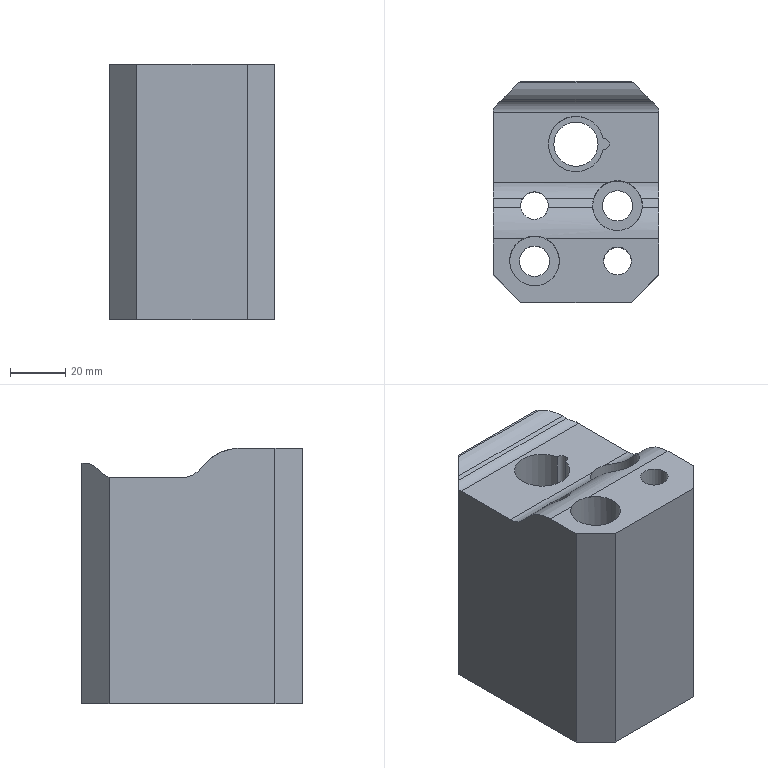Part | NX | features solid 2 | 1 solid | 35 faces | box 60 x 80 x 92.308 mm | volume 320475 mm3 | plane 20 | cylinder 15 | commonest cylinder face diameters 16 x4 10 x3 11 x2 18 x2 4 x1 20 x1
STEP:
#1=CARTESIAN_POINT('',(20.,-440.,5.));
#2=VERTEX_POINT('',#1);
#3=CARTESIAN_POINT('',(20.,-440.,97.308));
#4=VERTEX_POINT('',#3);
#5=CARTESIAN_POINT('',(20.,-440.,10.));
#6=DIRECTION('',(0.,0.,1.));
#7=VECTOR('',#6,1000.);
#8=LINE('',#5,#7);
#9=EDGE_CURVE('',#2,#4,#8,.T.);
#10=ORIENTED_EDGE('',*,*,#9,.T.);
#11=CARTESIAN_POINT('',(-20.,-440.,97.308));
#12=VERTEX_POINT('',#11);
#13=CARTESIAN_POINT('',(0.,-440.,97.308));
#14=DIRECTION('',(-1.,0.,0.));
#15=VECTOR('',#14,1000.);
#16=LINE('',#13,#15);
#17=EDGE_CURVE('',#4,#12,#16,.T.);
#18=ORIENTED_EDGE('',*,*,#17,.T.);
#19=CARTESIAN_POINT('',(-20.,-440.,5.));
#20=VERTEX_POINT('',#19);
#21=CARTESIAN_POINT('',(-20.,-440.,10.));
#22=DIRECTION('',(0.,0.,-1.));
#23=VECTOR('',#22,1000.);
#24=LINE('',#21,#23);
#25=EDGE_CURVE('',#12,#20,#24,.T.);
#26=ORIENTED_EDGE('',*,*,#25,.T.);
#27=CARTESIAN_POINT('',(0.,-440.,5.));
#28=DIRECTION('',(1.,0.,0.));
#29=VECTOR('',#28,1000.);
#30=LINE('',#27,#29);
#31=EDGE_CURVE('',#20,#2,#30,.T.);
#32=ORIENTED_EDGE('',*,*,#31,.T.);
#33=EDGE_LOOP('',(#10,#18,#26,#32));
#34=FACE_BOUND('',#33,.T.);
#35=CARTESIAN_POINT('',(0.,-440.,10.));
#36=DIRECTION('',(0.,-1.,0.));
#37=DIRECTION('',(0.,0.,-1.));
#38=AXIS2_PLACEMENT_3D('',#35,#36,#37);
#39=PLANE('',#38);
#40=ADVANCED_FACE('',(#34),#39,.T.);
#41=CARTESIAN_POINT('',(-20.,-360.,5.));
#42=VERTEX_POINT('',#41);
#43=CARTESIAN_POINT('',(-20.,-360.,92.008));
#44=VERTEX_POINT('',#43);
#45=CARTESIAN_POINT('',(-20.,-360.,10.));
#46=DIRECTION('',(0.,0.,1.));
#47=VECTOR('',#46,1000.);
#48=LINE('',#45,#47);
#49=EDGE_CURVE('',#42,#44,#48,.T.);
#50=ORIENTED_EDGE('',*,*,#49,.T.);
#51=CARTESIAN_POINT('',(20.,-360.,92.008));
#52=VERTEX_POINT('',#51);
#53=CARTESIAN_POINT('',(0.,-360.,92.008));
#54=DIRECTION('',(1.,0.,0.));
#55=VECTOR('',#54,1000.);
#56=LINE('',#53,#55);
#57=EDGE_CURVE('',#44,#52,#56,.T.);
#58=ORIENTED_EDGE('',*,*,#57,.T.);
#59=CARTESIAN_POINT('',(20.,-360.,5.));
#60=VERTEX_POINT('',#59);
#61=CARTESIAN_POINT('',(20.,-360.,10.));
#62=DIRECTION('',(0.,0.,-1.));
#63=VECTOR('',#62,1000.);
#64=LINE('',#61,#63);
#65=EDGE_CURVE('',#52,#60,#64,.T.);
#66=ORIENTED_EDGE('',*,*,#65,.T.);
#67=CARTESIAN_POINT('',(0.,-360.,5.));
#68=DIRECTION('',(-1.,0.,0.));
#69=VECTOR('',#68,1000.);
#70=LINE('',#67,#69);
#71=EDGE_CURVE('',#60,#42,#70,.T.);
#72=ORIENTED_EDGE('',*,*,#71,.T.);
#73=EDGE_LOOP('',(#50,#58,#66,#72));
#74=FACE_BOUND('',#73,.T.);
#75=CARTESIAN_POINT('',(0.,-360.,10.));
#76=DIRECTION('',(0.,1.,0.));
#77=DIRECTION('',(0.,0.,1.));
#78=AXIS2_PLACEMENT_3D('',#75,#76,#77);
#79=PLANE('',#78);
#80=ADVANCED_FACE('',(#74),#79,.T.);
#81=CARTESIAN_POINT('',(30.,-430.,97.308));
#82=VERTEX_POINT('',#81);
#83=CARTESIAN_POINT('',(30.,-430.,5.));
#84=VERTEX_POINT('',#83);
#85=CARTESIAN_POINT('',(30.,-430.,10.));
#86=DIRECTION('',(0.,0.,-1.));
#87=VECTOR('',#86,1000.);
#88=LINE('',#85,#87);
#89=EDGE_CURVE('',#82,#84,#88,.T.);
#90=ORIENTED_EDGE('',*,*,#89,.F.);
#91=CARTESIAN_POINT('',(20.,-440.,97.308));
#92=DIRECTION('',(0.7071,0.7071,0.));
#93=VECTOR('',#92,1000.);
#94=LINE('',#91,#93);
#95=EDGE_CURVE('',#82,#4,#94,.F.);
#96=ORIENTED_EDGE('',*,*,#95,.T.);
#97=ORIENTED_EDGE('',*,*,#9,.F.);
#98=CARTESIAN_POINT('',(50.,-410.,5.));
#99=DIRECTION('',(0.7071,0.7071,0.));
#100=VECTOR('',#99,1000.);
#101=LINE('',#98,#100);
#102=EDGE_CURVE('',#84,#2,#101,.F.);
#103=ORIENTED_EDGE('',*,*,#102,.F.);
#104=EDGE_LOOP('',(#90,#96,#97,#103));
#105=FACE_BOUND('',#104,.T.);
#106=CARTESIAN_POINT('',(20.,-440.,10.));
#107=DIRECTION('',(-0.7071,0.7071,0.));
#108=DIRECTION('',(-0.7071,-0.7071,0.));
#109=AXIS2_PLACEMENT_3D('',#106,#107,#108);
#110=PLANE('',#109);
#111=ADVANCED_FACE('',(#105),#110,.F.);
#112=ORIENTED_EDGE('',*,*,#25,.F.);
#113=CARTESIAN_POINT('',(-30.,-430.,97.308));
#114=VERTEX_POINT('',#113);
#115=CARTESIAN_POINT('',(-30.,-430.,97.308));
#116=DIRECTION('',(0.7071,-0.7071,0.));
#117=VECTOR('',#116,1000.);
#118=LINE('',#115,#117);
#119=EDGE_CURVE('',#12,#114,#118,.F.);
#120=ORIENTED_EDGE('',*,*,#119,.T.);
#121=CARTESIAN_POINT('',(-30.,-430.,5.));
#122=VERTEX_POINT('',#121);
#123=CARTESIAN_POINT('',(-30.,-430.,10.));
#124=DIRECTION('',(0.,0.,1.));
#125=VECTOR('',#124,1000.);
#126=LINE('',#123,#125);
#127=EDGE_CURVE('',#122,#114,#126,.T.);
#128=ORIENTED_EDGE('',*,*,#127,.F.);
#129=CARTESIAN_POINT('',(-50.,-410.,5.));
#130=DIRECTION('',(0.7071,-0.7071,0.));
#131=VECTOR('',#130,1000.);
#132=LINE('',#129,#131);
#133=EDGE_CURVE('',#20,#122,#132,.F.);
#134=ORIENTED_EDGE('',*,*,#133,.F.);
#135=EDGE_LOOP('',(#112,#120,#128,#134));
#136=FACE_BOUND('',#135,.T.);
#137=CARTESIAN_POINT('',(-30.,-430.,10.));
#138=DIRECTION('',(0.7071,0.7071,0.));
#139=DIRECTION('',(-0.7071,0.7071,0.));
#140=AXIS2_PLACEMENT_3D('',#137,#138,#139);
#141=PLANE('',#140);
#142=ADVANCED_FACE('',(#136),#141,.F.);
#143=CARTESIAN_POINT('',(10.,-425.,5.));
#144=VERTEX_POINT('',#143);
#145=CARTESIAN_POINT('',(15.,-425.,5.));
#146=DIRECTION('',(0.,0.,-1.));
#147=DIRECTION('',(-1.,0.,0.));
#148=AXIS2_PLACEMENT_3D('',#145,#146,#147);
#149=CIRCLE('',#148,5.);
#150=EDGE_CURVE('',#144,#144,#149,.T.);
#151=ORIENTED_EDGE('',*,*,#150,.T.);
#152=EDGE_LOOP('',(#151));
#153=FACE_BOUND('',#152,.T.);
#154=CARTESIAN_POINT('',(20.,-425.,97.308));
#155=VERTEX_POINT('',#154);
#156=CARTESIAN_POINT('',(15.,-425.,97.308));
#157=DIRECTION('',(0.,0.,1.));
#158=DIRECTION('',(1.,0.,0.));
#159=AXIS2_PLACEMENT_3D('',#156,#157,#158);
#160=CIRCLE('',#159,5.);
#161=EDGE_CURVE('',#155,#155,#160,.F.);
#162=ORIENTED_EDGE('',*,*,#161,.F.);
#163=EDGE_LOOP('',(#162));
#164=FACE_BOUND('',#163,.T.);
#165=CARTESIAN_POINT('',(15.,-425.,110.));
#166=DIRECTION('',(0.,0.,-1.));
#167=DIRECTION('',(-1.,0.,0.));
#168=AXIS2_PLACEMENT_3D('',#165,#166,#167);
#169=CYLINDRICAL_SURFACE('',#168,5.);
#170=ADVANCED_FACE('',(#153,#164),#169,.F.);
#171=CARTESIAN_POINT('',(-24.,-425.,35.));
#172=VERTEX_POINT('',#171);
#173=CARTESIAN_POINT('',(-15.,-425.,35.));
#174=DIRECTION('',(0.,0.,-1.));
#175=DIRECTION('',(-1.,0.,0.));
#176=AXIS2_PLACEMENT_3D('',#173,#174,#175);
#177=CIRCLE('',#176,9.);
#178=EDGE_CURVE('',#172,#172,#177,.T.);
#179=ORIENTED_EDGE('',*,*,#178,.T.);
#180=EDGE_LOOP('',(#179));
#181=FACE_BOUND('',#180,.T.);
#182=CARTESIAN_POINT('',(-10.799,-417.041,97.308));
#183=VERTEX_POINT('',#182);
#184=CARTESIAN_POINT('',(-19.201,-417.041,97.308));
#185=VERTEX_POINT('',#184);
#186=CARTESIAN_POINT('',(-15.,-425.,97.308));
#187=DIRECTION('',(0.,0.,1.));
#188=DIRECTION('',(1.,0.,0.));
#189=AXIS2_PLACEMENT_3D('',#186,#187,#188);
#190=CIRCLE('',#189,9.);
#191=EDGE_CURVE('',#183,#185,#190,.F.);
#192=ORIENTED_EDGE('',*,*,#191,.F.);
#193=CARTESIAN_POINT('',(-19.201,-417.041,97.308));
#194=CARTESIAN_POINT('',(-17.901,-416.354,97.308));
#195=CARTESIAN_POINT('',(-15.004,-415.646,97.24));
#196=CARTESIAN_POINT('',(-12.099,-416.354,97.308));
#197=CARTESIAN_POINT('',(-10.799,-417.041,97.308));
#198=B_SPLINE_CURVE_WITH_KNOTS('',3,(#193,#194,#195,#196,#197),.UNSPECIFIED.,.F.,.F.,(4,1,4),(0.,0.004347,0.008695),.UNSPECIFIED.);
#199=EDGE_CURVE('',#185,#183,#198,.T.);
#200=ORIENTED_EDGE('',*,*,#199,.F.);
#201=EDGE_LOOP('',(#192,#200));
#202=FACE_BOUND('',#201,.T.);
#203=CARTESIAN_POINT('',(-15.,-425.,110.));
#204=DIRECTION('',(0.,0.,-1.));
#205=DIRECTION('',(-1.,0.,0.));
#206=AXIS2_PLACEMENT_3D('',#203,#204,#205);
#207=CYLINDRICAL_SURFACE('',#206,9.);
#208=ADVANCED_FACE('',(#181,#202),#207,.F.);
#209=CARTESIAN_POINT('',(-30.,-370.,86.857));
#210=VERTEX_POINT('',#209);
#211=CARTESIAN_POINT('',(-30.,-371.212,86.708));
#212=VERTEX_POINT('',#211);
#213=CARTESIAN_POINT('',(-30.,-371.212,91.708));
#214=DIRECTION('',(-1.,0.,0.));
#215=DIRECTION('',(0.,0.,1.));
#216=AXIS2_PLACEMENT_3D('',#213,#214,#215);
#217=CIRCLE('',#216,5.);
#218=EDGE_CURVE('',#210,#212,#217,.T.);
#219=ORIENTED_EDGE('',*,*,#218,.F.);
#220=CARTESIAN_POINT('',(-30.,-370.,5.));
#221=VERTEX_POINT('',#220);
#222=CARTESIAN_POINT('',(-30.,-370.,10.));
#223=DIRECTION('',(0.,0.,-1.));
#224=VECTOR('',#223,1000.);
#225=LINE('',#222,#224);
#226=EDGE_CURVE('',#210,#221,#225,.T.);
#227=ORIENTED_EDGE('',*,*,#226,.T.);
#228=CARTESIAN_POINT('',(-30.,-360.,5.));
#229=DIRECTION('',(0.,-1.,0.));
#230=VECTOR('',#229,1000.);
#231=LINE('',#228,#230);
#232=EDGE_CURVE('',#221,#122,#231,.T.);
#233=ORIENTED_EDGE('',*,*,#232,.T.);
#234=ORIENTED_EDGE('',*,*,#127,.T.);
#235=CARTESIAN_POINT('',(-30.,-417.041,97.308));
#236=VERTEX_POINT('',#235);
#237=CARTESIAN_POINT('',(-30.,-360.,97.308));
#238=DIRECTION('',(0.,1.,0.));
#239=VECTOR('',#238,1000.);
#240=LINE('',#237,#239);
#241=EDGE_CURVE('',#114,#236,#240,.T.);
#242=ORIENTED_EDGE('',*,*,#241,.T.);
#243=CARTESIAN_POINT('',(-30.,-405.652,92.546));
#244=VERTEX_POINT('',#243);
#245=CARTESIAN_POINT('',(-30.,-417.041,81.308));
#246=DIRECTION('',(-1.,0.,0.));
#247=DIRECTION('',(0.,0.,1.));
#248=AXIS2_PLACEMENT_3D('',#245,#246,#247);
#249=CIRCLE('',#248,16.);
#250=EDGE_CURVE('',#236,#244,#249,.T.);
#251=ORIENTED_EDGE('',*,*,#250,.T.);
#252=CARTESIAN_POINT('',(-30.,-402.24,89.089));
#253=VERTEX_POINT('',#252);
#254=CARTESIAN_POINT('',(-30.,-341.861,27.899));
#255=DIRECTION('',(0.,-0.7024,0.7118));
#256=VECTOR('',#255,1000.);
#257=LINE('',#254,#256);
#258=EDGE_CURVE('',#253,#244,#257,.T.);
#259=ORIENTED_EDGE('',*,*,#258,.F.);
#260=CARTESIAN_POINT('',(-30.,-396.546,86.708));
#261=VERTEX_POINT('',#260);
#262=CARTESIAN_POINT('',(-30.,-396.546,94.708));
#263=DIRECTION('',(-1.,0.,0.));
#264=DIRECTION('',(0.,0.,1.));
#265=AXIS2_PLACEMENT_3D('',#262,#263,#264);
#266=CIRCLE('',#265,8.);
#267=EDGE_CURVE('',#261,#253,#266,.T.);
#268=ORIENTED_EDGE('',*,*,#267,.F.);
#269=CARTESIAN_POINT('',(-30.,-360.,86.708));
#270=DIRECTION('',(0.,1.,0.));
#271=VECTOR('',#270,1000.);
#272=LINE('',#269,#271);
#273=EDGE_CURVE('',#261,#212,#272,.T.);
#274=ORIENTED_EDGE('',*,*,#273,.T.);
#275=EDGE_LOOP('',(#219,#227,#233,#234,#242,#251,#259,#268,#274));
#276=FACE_BOUND('',#275,.T.);
#277=CARTESIAN_POINT('',(-30.,-360.,10.));
#278=DIRECTION('',(-1.,0.,0.));
#279=DIRECTION('',(0.,0.,1.));
#280=AXIS2_PLACEMENT_3D('',#277,#278,#279);
#281=PLANE('',#280);
#282=ADVANCED_FACE('',(#276),#281,.T.);
#283=CARTESIAN_POINT('',(-11.511,-382.714,5.));
#284=VERTEX_POINT('',#283);
#285=CARTESIAN_POINT('',(-0.01051,-382.714,5.));
#286=DIRECTION('',(0.,0.,-1.));
#287=DIRECTION('',(-1.,0.,0.));
#288=AXIS2_PLACEMENT_3D('',#285,#286,#287);
#289=CIRCLE('',#288,11.5);
#290=EDGE_CURVE('',#284,#284,#289,.F.);
#291=ORIENTED_EDGE('',*,*,#290,.T.);
#292=EDGE_LOOP('',(#291));
#293=FACE_BOUND('',#292,.T.);
#294=CARTESIAN_POINT('',(9.5,-405.,5.));
#295=VERTEX_POINT('',#294);
#296=CARTESIAN_POINT('',(15.,-405.,5.));
#297=DIRECTION('',(0.,0.,-1.));
#298=DIRECTION('',(-1.,0.,0.));
#299=AXIS2_PLACEMENT_3D('',#296,#297,#298);
#300=CIRCLE('',#299,5.5);
#301=EDGE_CURVE('',#295,#295,#300,.T.);
#302=ORIENTED_EDGE('',*,*,#301,.F.);
#303=EDGE_LOOP('',(#302));
#304=FACE_BOUND('',#303,.T.);
#305=CARTESIAN_POINT('',(-20.5,-425.,5.));
#306=VERTEX_POINT('',#305);
#307=CARTESIAN_POINT('',(-15.,-425.,5.));
#308=DIRECTION('',(0.,0.,-1.));
#309=DIRECTION('',(-1.,0.,0.));
#310=AXIS2_PLACEMENT_3D('',#307,#308,#309);
#311=CIRCLE('',#310,5.5);
#312=EDGE_CURVE('',#306,#306,#311,.T.);
#313=ORIENTED_EDGE('',*,*,#312,.F.);
#314=EDGE_LOOP('',(#313));
#315=FACE_BOUND('',#314,.T.);
#316=CARTESIAN_POINT('',(-20.,-405.,5.));
#317=VERTEX_POINT('',#316);
#318=CARTESIAN_POINT('',(-15.,-405.,5.));
#319=DIRECTION('',(0.,0.,-1.));
#320=DIRECTION('',(-1.,0.,0.));
#321=AXIS2_PLACEMENT_3D('',#318,#319,#320);
#322=CIRCLE('',#321,5.);
#323=EDGE_CURVE('',#317,#317,#322,.T.);
#324=ORIENTED_EDGE('',*,*,#323,.F.);
#325=EDGE_LOOP('',(#324));
#326=FACE_BOUND('',#325,.T.);
#327=ORIENTED_EDGE('',*,*,#150,.F.);
#328=EDGE_LOOP('',(#327));
#329=FACE_BOUND('',#328,.T.);
#330=CARTESIAN_POINT('',(30.,-370.,5.));
#331=VERTEX_POINT('',#330);
#332=CARTESIAN_POINT('',(30.,-360.,5.));
#333=DIRECTION('',(0.,1.,0.));
#334=VECTOR('',#333,1000.);
#335=LINE('',#332,#334);
#336=EDGE_CURVE('',#84,#331,#335,.T.);
#337=ORIENTED_EDGE('',*,*,#336,.F.);
#338=ORIENTED_EDGE('',*,*,#102,.T.);
#339=ORIENTED_EDGE('',*,*,#31,.F.);
#340=ORIENTED_EDGE('',*,*,#133,.T.);
#341=ORIENTED_EDGE('',*,*,#232,.F.);
#342=CARTESIAN_POINT('',(-10.,-350.,5.));
#343=DIRECTION('',(-0.7071,-0.7071,0.));
#344=VECTOR('',#343,1000.);
#345=LINE('',#342,#344);
#346=EDGE_CURVE('',#221,#42,#345,.F.);
#347=ORIENTED_EDGE('',*,*,#346,.T.);
#348=ORIENTED_EDGE('',*,*,#71,.F.);
#349=CARTESIAN_POINT('',(10.,-350.,5.));
#350=DIRECTION('',(-0.7071,0.7071,0.));
#351=VECTOR('',#350,1000.);
#352=LINE('',#349,#351);
#353=EDGE_CURVE('',#60,#331,#352,.F.);
#354=ORIENTED_EDGE('',*,*,#353,.T.);
#355=EDGE_LOOP('',(#337,#338,#339,#340,#341,#347,#348,#354));
#356=FACE_BOUND('',#355,.T.);
#357=CARTESIAN_POINT('',(0.,-360.,5.));
#358=DIRECTION('',(0.,0.,-1.));
#359=DIRECTION('',(-1.,0.,0.));
#360=AXIS2_PLACEMENT_3D('',#357,#358,#359);
#361=PLANE('',#360);
#362=ADVANCED_FACE('',(#293,#304,#315,#326,#329,#356),#361,.T.);
#363=CARTESIAN_POINT('',(30.,-371.212,86.708));
#364=VERTEX_POINT('',#363);
#365=CARTESIAN_POINT('',(30.,-370.,86.857));
#366=VERTEX_POINT('',#365);
#367=CARTESIAN_POINT('',(30.,-371.212,91.708));
#368=DIRECTION('',(1.,0.,0.));
#369=DIRECTION('',(0.,0.,-1.));
#370=AXIS2_PLACEMENT_3D('',#367,#368,#369);
#371=CIRCLE('',#370,5.);
#372=EDGE_CURVE('',#364,#366,#371,.T.);
#373=ORIENTED_EDGE('',*,*,#372,.F.);
#374=CARTESIAN_POINT('',(30.,-396.546,86.708));
#375=VERTEX_POINT('',#374);
#376=CARTESIAN_POINT('',(30.,-360.,86.708));
#377=DIRECTION('',(0.,-1.,0.));
#378=VECTOR('',#377,1000.);
#379=LINE('',#376,#378);
#380=EDGE_CURVE('',#364,#375,#379,.T.);
#381=ORIENTED_EDGE('',*,*,#380,.T.);
#382=CARTESIAN_POINT('',(30.,-402.24,89.089));
#383=VERTEX_POINT('',#382);
#384=CARTESIAN_POINT('',(30.,-396.546,94.708));
#385=DIRECTION('',(1.,0.,0.));
#386=DIRECTION('',(0.,0.,-1.));
#387=AXIS2_PLACEMENT_3D('',#384,#385,#386);
#388=CIRCLE('',#387,8.);
#389=EDGE_CURVE('',#383,#375,#388,.T.);
#390=ORIENTED_EDGE('',*,*,#389,.F.);
#391=CARTESIAN_POINT('',(30.,-405.652,92.546));
#392=VERTEX_POINT('',#391);
#393=CARTESIAN_POINT('',(30.,-341.861,27.899));
#394=DIRECTION('',(0.,0.7024,-0.7118));
#395=VECTOR('',#394,1000.);
#396=LINE('',#393,#395);
#397=EDGE_CURVE('',#392,#383,#396,.T.);
#398=ORIENTED_EDGE('',*,*,#397,.F.);
#399=CARTESIAN_POINT('',(30.,-417.041,97.308));
#400=VERTEX_POINT('',#399);
#401=CARTESIAN_POINT('',(30.,-417.041,81.308));
#402=DIRECTION('',(1.,0.,0.));
#403=DIRECTION('',(0.,0.,-1.));
#404=AXIS2_PLACEMENT_3D('',#401,#402,#403);
#405=CIRCLE('',#404,16.);
#406=EDGE_CURVE('',#392,#400,#405,.T.);
#407=ORIENTED_EDGE('',*,*,#406,.T.);
#408=CARTESIAN_POINT('',(30.,-360.,97.308));
#409=DIRECTION('',(0.,-1.,0.));
#410=VECTOR('',#409,1000.);
#411=LINE('',#408,#410);
#412=EDGE_CURVE('',#400,#82,#411,.T.);
#413=ORIENTED_EDGE('',*,*,#412,.T.);
#414=ORIENTED_EDGE('',*,*,#89,.T.);
#415=ORIENTED_EDGE('',*,*,#336,.T.);
#416=CARTESIAN_POINT('',(30.,-370.,10.));
#417=DIRECTION('',(0.,0.,1.));
#418=VECTOR('',#417,1000.);
#419=LINE('',#416,#418);
#420=EDGE_CURVE('',#331,#366,#419,.T.);
#421=ORIENTED_EDGE('',*,*,#420,.T.);
#422=EDGE_LOOP('',(#373,#381,#390,#398,#407,#413,#414,#415,#421));
#423=FACE_BOUND('',#422,.T.);
#424=CARTESIAN_POINT('',(30.,-360.,10.));
#425=DIRECTION('',(1.,0.,0.));
#426=DIRECTION('',(0.,0.,-1.));
#427=AXIS2_PLACEMENT_3D('',#424,#425,#426);
#428=PLANE('',#427);
#429=ADVANCED_FACE('',(#423),#428,.T.);
#430=CARTESIAN_POINT('',(27.512,-367.512,88.345));
#431=VERTEX_POINT('',#430);
#432=CARTESIAN_POINT('',(31.212,-371.212,91.708));
#433=DIRECTION('',(-0.7071,-0.7071,0.));
#434=DIRECTION('',(-0.7071,0.7071,0.));
#435=AXIS2_PLACEMENT_3D('',#432,#433,#434);
#436=ELLIPSE('',#435,7.071,5.);
#437=EDGE_CURVE('',#366,#431,#436,.F.);
#438=ORIENTED_EDGE('',*,*,#437,.F.);
#439=ORIENTED_EDGE('',*,*,#420,.F.);
#440=ORIENTED_EDGE('',*,*,#353,.F.);
#441=ORIENTED_EDGE('',*,*,#65,.F.);
#442=CARTESIAN_POINT('',(20.643,-360.643,92.008));
#443=VERTEX_POINT('',#442);
#444=CARTESIAN_POINT('',(30.,-370.,92.008));
#445=DIRECTION('',(-0.7071,0.7071,0.));
#446=VECTOR('',#445,1000.);
#447=LINE('',#444,#446);
#448=EDGE_CURVE('',#52,#443,#447,.F.);
#449=ORIENTED_EDGE('',*,*,#448,.T.);
#450=CARTESIAN_POINT('',(26.564,-366.564,89.388));
#451=VERTEX_POINT('',#450);
#452=CARTESIAN_POINT('',(20.643,-360.643,84.008));
#453=DIRECTION('',(-0.7071,-0.7071,0.));
#454=DIRECTION('',(-0.7071,0.7071,0.));
#455=AXIS2_PLACEMENT_3D('',#452,#453,#454);
#456=ELLIPSE('',#455,11.314,8.);
#457=EDGE_CURVE('',#443,#451,#456,.F.);
#458=ORIENTED_EDGE('',*,*,#457,.T.);
#459=CARTESIAN_POINT('',(55.911,-395.911,57.099));
#460=DIRECTION('',(-0.5581,0.5581,0.614));
#461=VECTOR('',#460,1000.);
#462=LINE('',#459,#461);
#463=EDGE_CURVE('',#451,#431,#462,.F.);
#464=ORIENTED_EDGE('',*,*,#463,.T.);
#465=EDGE_LOOP('',(#438,#439,#440,#441,#449,#458,#464));
#466=FACE_BOUND('',#465,.T.);
#467=CARTESIAN_POINT('',(30.,-370.,10.));
#468=DIRECTION('',(-0.7071,-0.7071,0.));
#469=DIRECTION('',(0.7071,-0.7071,0.));
#470=AXIS2_PLACEMENT_3D('',#467,#468,#469);
#471=PLANE('',#470);
#472=ADVANCED_FACE('',(#466),#471,.F.);
#473=CARTESIAN_POINT('',(-27.512,-367.512,88.345));
#474=VERTEX_POINT('',#473);
#475=CARTESIAN_POINT('',(-31.212,-371.212,91.708));
#476=DIRECTION('',(0.7071,-0.7071,0.));
#477=DIRECTION('',(-0.7071,-0.7071,0.));
#478=AXIS2_PLACEMENT_3D('',#475,#476,#477);
#479=ELLIPSE('',#478,7.071,5.);
#480=EDGE_CURVE('',#474,#210,#479,.F.);
#481=ORIENTED_EDGE('',*,*,#480,.F.);
#482=CARTESIAN_POINT('',(-26.564,-366.564,89.388));
#483=VERTEX_POINT('',#482);
#484=CARTESIAN_POINT('',(-49.681,-389.681,63.953));
#485=DIRECTION('',(-0.5581,-0.5581,-0.614));
#486=VECTOR('',#485,1000.);
#487=LINE('',#484,#486);
#488=EDGE_CURVE('',#474,#483,#487,.F.);
#489=ORIENTED_EDGE('',*,*,#488,.T.);
#490=CARTESIAN_POINT('',(-20.643,-360.643,92.008));
#491=VERTEX_POINT('',#490);
#492=CARTESIAN_POINT('',(-20.643,-360.643,84.008));
#493=DIRECTION('',(0.7071,-0.7071,0.));
#494=DIRECTION('',(-0.7071,-0.7071,0.));
#495=AXIS2_PLACEMENT_3D('',#492,#493,#494);
#496=ELLIPSE('',#495,11.314,8.);
#497=EDGE_CURVE('',#483,#491,#496,.F.);
#498=ORIENTED_EDGE('',*,*,#497,.T.);
#499=CARTESIAN_POINT('',(-20.,-360.,92.008));
#500=DIRECTION('',(-0.7071,-0.7071,0.));
#501=VECTOR('',#500,1000.);
#502=LINE('',#499,#501);
#503=EDGE_CURVE('',#491,#44,#502,.F.);
#504=ORIENTED_EDGE('',*,*,#503,.T.);
#505=ORIENTED_EDGE('',*,*,#49,.F.);
#506=ORIENTED_EDGE('',*,*,#346,.F.);
#507=ORIENTED_EDGE('',*,*,#226,.F.);
#508=EDGE_LOOP('',(#481,#489,#498,#504,#505,#506,#507));
#509=FACE_BOUND('',#508,.T.);
#510=CARTESIAN_POINT('',(-20.,-360.,10.));
#511=DIRECTION('',(0.7071,-0.7071,0.));
#512=DIRECTION('',(0.7071,0.7071,0.));
#513=AXIS2_PLACEMENT_3D('',#510,#511,#512);
#514=PLANE('',#513);
#515=ADVANCED_FACE('',(#509),#514,.F.);
#516=CARTESIAN_POINT('',(-10.831,-402.24,89.089));
#517=VERTEX_POINT('',#516);
#518=CARTESIAN_POINT('',(-19.169,-402.24,89.089));
#519=VERTEX_POINT('',#518);
#520=CARTESIAN_POINT('',(-10.831,-402.24,89.089));
#521=CARTESIAN_POINT('',(-11.206,-401.674,88.514));
#522=CARTESIAN_POINT('',(-12.345,-400.5,87.7));
#523=CARTESIAN_POINT('',(-15.,-399.751,87.388));
#524=CARTESIAN_POINT('',(-17.652,-400.498,87.699));
#525=CARTESIAN_POINT('',(-18.794,-401.674,88.514));
#526=CARTESIAN_POINT('',(-19.169,-402.24,89.089));
#527=B_SPLINE_CURVE_WITH_KNOTS('',3,(#520,#521,#522,#523,#524,#525,#526),.UNSPECIFIED.,.F.,.F.,(4,1,1,1,4),(0.,0.002634,0.005268,0.007902,0.01054),.UNSPECIFIED.);
#528=EDGE_CURVE('',#517,#519,#527,.T.);
#529=ORIENTED_EDGE('',*,*,#528,.T.);
#530=CARTESIAN_POINT('',(-19.957,-405.652,92.546));
#531=VERTEX_POINT('',#530);
#532=CARTESIAN_POINT('',(-15.,-405.,91.885));
#533=DIRECTION('',(0.,-0.7118,-0.7024));
#534=DIRECTION('',(0.,0.7024,-0.7118));
#535=AXIS2_PLACEMENT_3D('',#532,#533,#534);
#536=ELLIPSE('',#535,7.119,5.);
#537=EDGE_CURVE('',#519,#531,#536,.F.);
#538=ORIENTED_EDGE('',*,*,#537,.T.);
#539=CARTESIAN_POINT('',(-10.043,-405.652,92.546));
#540=VERTEX_POINT('',#539);
#541=CARTESIAN_POINT('',(-10.043,-405.652,92.546));
#542=CARTESIAN_POINT('',(-10.167,-406.597,93.504));
#543=CARTESIAN_POINT('',(-11.003,-408.762,95.124));
#544=CARTESIAN_POINT('',(-14.989,-410.615,95.949));
#545=CARTESIAN_POINT('',(-18.985,-408.779,95.134));
#546=CARTESIAN_POINT('',(-19.833,-406.599,93.506));
#547=CARTESIAN_POINT('',(-19.957,-405.652,92.546));
#548=B_SPLINE_CURVE_WITH_KNOTS('',3,(#541,#542,#543,#544,#545,#546,#547),.UNSPECIFIED.,.F.,.F.,(4,1,1,1,4),(0.,0.003993,0.007986,0.01198,0.01597),.UNSPECIFIED.);
#549=EDGE_CURVE('',#540,#531,#548,.T.);
#550=ORIENTED_EDGE('',*,*,#549,.F.);
#551=CARTESIAN_POINT('',(-15.,-405.,91.885));
#552=DIRECTION('',(0.,-0.7118,-0.7024));
#553=DIRECTION('',(0.,0.7024,-0.7118));
#554=AXIS2_PLACEMENT_3D('',#551,#552,#553);
#555=ELLIPSE('',#554,7.119,5.);
#556=EDGE_CURVE('',#540,#517,#555,.F.);
#557=ORIENTED_EDGE('',*,*,#556,.T.);
#558=EDGE_LOOP('',(#529,#538,#550,#557));
#559=FACE_BOUND('',#558,.T.);
#560=ORIENTED_EDGE('',*,*,#323,.T.);
#561=EDGE_LOOP('',(#560));
#562=FACE_BOUND('',#561,.T.);
#563=CARTESIAN_POINT('',(-15.,-405.,110.));
#564=DIRECTION('',(0.,0.,-1.));
#565=DIRECTION('',(-1.,0.,0.));
#566=AXIS2_PLACEMENT_3D('',#563,#564,#565);
#567=CYLINDRICAL_SURFACE('',#566,5.);
#568=ADVANCED_FACE('',(#559,#562),#567,.F.);
#569=ORIENTED_EDGE('',*,*,#312,.T.);
#570=EDGE_LOOP('',(#569));
#571=FACE_BOUND('',#570,.T.);
#572=CARTESIAN_POINT('',(-20.5,-425.,35.));
#573=VERTEX_POINT('',#572);
#574=CARTESIAN_POINT('',(-15.,-425.,35.));
#575=DIRECTION('',(0.,0.,-1.));
#576=DIRECTION('',(-1.,0.,0.));
#577=AXIS2_PLACEMENT_3D('',#574,#575,#576);
#578=CIRCLE('',#577,5.5);
#579=EDGE_CURVE('',#573,#573,#578,.T.);
#580=ORIENTED_EDGE('',*,*,#579,.F.);
#581=EDGE_LOOP('',(#580));
#582=FACE_BOUND('',#581,.T.);
#583=CARTESIAN_POINT('',(-15.,-425.,5.));
#584=DIRECTION('',(0.,0.,-1.));
#585=DIRECTION('',(-1.,0.,0.));
#586=AXIS2_PLACEMENT_3D('',#583,#584,#585);
#587=CYLINDRICAL_SURFACE('',#586,5.5);
#588=ADVANCED_FACE('',(#571,#582),#587,.F.);
#589=ORIENTED_EDGE('',*,*,#579,.T.);
#590=EDGE_LOOP('',(#589));
#591=FACE_BOUND('',#590,.T.);
#592=ORIENTED_EDGE('',*,*,#178,.F.);
#593=EDGE_LOOP('',(#592));
#594=FACE_BOUND('',#593,.T.);
#595=CARTESIAN_POINT('',(-15.,-425.,35.));
#596=DIRECTION('',(0.,0.,-1.));
#597=DIRECTION('',(-1.,0.,0.));
#598=AXIS2_PLACEMENT_3D('',#595,#596,#597);
#599=PLANE('',#598);
#600=ADVANCED_FACE('',(#591,#594),#599,.F.);
#601=ORIENTED_EDGE('',*,*,#301,.T.);
#602=EDGE_LOOP('',(#601));
#603=FACE_BOUND('',#602,.T.);
#604=CARTESIAN_POINT('',(9.5,-405.,35.));
#605=VERTEX_POINT('',#604);
#606=CARTESIAN_POINT('',(15.,-405.,35.));
#607=DIRECTION('',(0.,0.,-1.));
#608=DIRECTION('',(-1.,0.,0.));
#609=AXIS2_PLACEMENT_3D('',#606,#607,#608);
#610=CIRCLE('',#609,5.5);
#611=EDGE_CURVE('',#605,#605,#610,.T.);
#612=ORIENTED_EDGE('',*,*,#611,.F.);
#613=EDGE_LOOP('',(#612));
#614=FACE_BOUND('',#613,.T.);
#615=CARTESIAN_POINT('',(15.,-405.,5.));
#616=DIRECTION('',(0.,0.,-1.));
#617=DIRECTION('',(-1.,0.,0.));
#618=AXIS2_PLACEMENT_3D('',#615,#616,#617);
#619=CYLINDRICAL_SURFACE('',#618,5.5);
#620=ADVANCED_FACE('',(#603,#614),#619,.F.);
#621=ORIENTED_EDGE('',*,*,#611,.T.);
#622=EDGE_LOOP('',(#621));
#623=FACE_BOUND('',#622,.T.);
#624=CARTESIAN_POINT('',(6.,-405.,35.));
#625=VERTEX_POINT('',#624);
#626=CARTESIAN_POINT('',(15.,-405.,35.));
#627=DIRECTION('',(0.,0.,-1.));
#628=DIRECTION('',(-1.,0.,0.));
#629=AXIS2_PLACEMENT_3D('',#626,#627,#628);
#630=CIRCLE('',#629,9.);
#631=EDGE_CURVE('',#625,#625,#630,.T.);
#632=ORIENTED_EDGE('',*,*,#631,.F.);
#633=EDGE_LOOP('',(#632));
#634=FACE_BOUND('',#633,.T.);
#635=CARTESIAN_POINT('',(15.,-405.,35.));
#636=DIRECTION('',(0.,0.,-1.));
#637=DIRECTION('',(-1.,0.,0.));
#638=AXIS2_PLACEMENT_3D('',#635,#636,#637);
#639=PLANE('',#638);
#640=ADVANCED_FACE('',(#623,#634),#639,.F.);
#641=CARTESIAN_POINT('',(11.913,-396.546,86.708));
#642=VERTEX_POINT('',#641);
#643=CARTESIAN_POINT('',(18.087,-396.546,86.708));
#644=VERTEX_POINT('',#643);
#645=CARTESIAN_POINT('',(15.,-405.,86.708));
#646=DIRECTION('',(0.,0.,1.));
#647=DIRECTION('',(1.,0.,0.));
#648=AXIS2_PLACEMENT_3D('',#645,#646,#647);
#649=CIRCLE('',#648,9.);
#650=EDGE_CURVE('',#642,#644,#649,.F.);
#651=ORIENTED_EDGE('',*,*,#650,.F.);
#652=CARTESIAN_POINT('',(6.434,-402.24,89.089));
#653=VERTEX_POINT('',#652);
#654=CARTESIAN_POINT('',(11.913,-396.546,86.708));
#655=CARTESIAN_POINT('',(10.531,-397.051,86.708));
#656=CARTESIAN_POINT('',(8.034,-398.754,86.767));
#657=CARTESIAN_POINT('',(6.759,-401.229,88.064));
#658=CARTESIAN_POINT('',(6.434,-402.24,89.089));
#659=B_SPLINE_CURVE_WITH_KNOTS('',3,(#654,#655,#656,#657,#658),.UNSPECIFIED.,.F.,.F.,(4,1,4),(0.,0.004358,0.008716),.UNSPECIFIED.);
#660=EDGE_CURVE('',#642,#653,#659,.T.);
#661=ORIENTED_EDGE('',*,*,#660,.T.);
#662=CARTESIAN_POINT('',(6.024,-405.652,92.546));
#663=VERTEX_POINT('',#662);
#664=CARTESIAN_POINT('',(15.,-405.,91.885));
#665=DIRECTION('',(0.,-0.7118,-0.7024));
#666=DIRECTION('',(0.,0.7024,-0.7118));
#667=AXIS2_PLACEMENT_3D('',#664,#665,#666);
#668=ELLIPSE('',#667,12.814,9.);
#669=EDGE_CURVE('',#653,#663,#668,.F.);
#670=ORIENTED_EDGE('',*,*,#669,.T.);
#671=CARTESIAN_POINT('',(23.976,-405.652,92.546));
#672=VERTEX_POINT('',#671);
#673=CARTESIAN_POINT('',(23.976,-405.652,92.546));
#674=CARTESIAN_POINT('',(23.914,-406.513,93.419));
#675=CARTESIAN_POINT('',(23.527,-408.421,94.941));
#676=CARTESIAN_POINT('',(21.701,-411.359,96.352));
#677=CARTESIAN_POINT('',(18.672,-413.492,96.93));
#678=CARTESIAN_POINT('',(15.017,-414.251,97.058));
#679=CARTESIAN_POINT('',(11.353,-413.503,96.933));
#680=CARTESIAN_POINT('',(8.315,-411.377,96.358));
#681=CARTESIAN_POINT('',(6.476,-408.434,94.95));
#682=CARTESIAN_POINT('',(6.086,-406.514,93.42));
#683=CARTESIAN_POINT('',(6.024,-405.652,92.546));
#684=B_SPLINE_CURVE_WITH_KNOTS('',3,(#673,#674,#675,#676,#677,#678,#679,#680,#681,#682,#683),.UNSPECIFIED.,.F.,.F.,(4,1,1,1,1,1,1,1,4),(0.,0.003639,0.007278,0.01092,0.01456,0.01819,0.02183,0.02547,0.02911),.UNSPECIFIED.);
#685=EDGE_CURVE('',#672,#663,#684,.T.);
#686=ORIENTED_EDGE('',*,*,#685,.F.);
#687=CARTESIAN_POINT('',(23.566,-402.24,89.089));
#688=VERTEX_POINT('',#687);
#689=CARTESIAN_POINT('',(15.,-405.,91.885));
#690=DIRECTION('',(0.,-0.7118,-0.7024));
#691=DIRECTION('',(0.,0.7024,-0.7118));
#692=AXIS2_PLACEMENT_3D('',#689,#690,#691);
#693=ELLIPSE('',#692,12.814,9.);
#694=EDGE_CURVE('',#672,#688,#693,.F.);
#695=ORIENTED_EDGE('',*,*,#694,.T.);
#696=CARTESIAN_POINT('',(23.566,-402.24,89.089));
#697=CARTESIAN_POINT('',(23.242,-401.232,88.067));
#698=CARTESIAN_POINT('',(21.982,-398.77,86.771));
#699=CARTESIAN_POINT('',(19.467,-397.05,86.708));
#700=CARTESIAN_POINT('',(18.087,-396.546,86.708));
#701=B_SPLINE_CURVE_WITH_KNOTS('',3,(#696,#697,#698,#699,#700),.UNSPECIFIED.,.F.,.F.,(4,1,4),(0.,0.004352,0.008704),.UNSPECIFIED.);
#702=EDGE_CURVE('',#688,#644,#701,.T.);
#703=ORIENTED_EDGE('',*,*,#702,.T.);
#704=EDGE_LOOP('',(#651,#661,#670,#686,#695,#703));
#705=FACE_BOUND('',#704,.T.);
#706=ORIENTED_EDGE('',*,*,#631,.T.);
#707=EDGE_LOOP('',(#706));
#708=FACE_BOUND('',#707,.T.);
#709=CARTESIAN_POINT('',(15.,-405.,110.));
#710=DIRECTION('',(0.,0.,-1.));
#711=DIRECTION('',(-1.,0.,0.));
#712=AXIS2_PLACEMENT_3D('',#709,#710,#711);
#713=CYLINDRICAL_SURFACE('',#712,9.);
#714=ADVANCED_FACE('',(#705,#708),#713,.F.);
#715=ORIENTED_EDGE('',*,*,#412,.F.);
#716=CARTESIAN_POINT('',(30.,-417.041,97.308));
#717=CARTESIAN_POINT('',(16.4,-417.041,97.308));
#718=CARTESIAN_POINT('',(2.801,-417.041,97.308));
#719=CARTESIAN_POINT('',(-10.799,-417.041,97.308));
#720=B_SPLINE_CURVE_WITH_KNOTS('',3,(#716,#717,#718,#719),.UNSPECIFIED.,.F.,.F.,(4,4),(0.4635,0.5128),.UNSPECIFIED.);
#721=EDGE_CURVE('',#400,#183,#720,.T.);
#722=ORIENTED_EDGE('',*,*,#721,.T.);
#723=ORIENTED_EDGE('',*,*,#191,.T.);
#724=CARTESIAN_POINT('',(-19.201,-417.041,97.308));
#725=CARTESIAN_POINT('',(-22.801,-417.041,97.308));
#726=CARTESIAN_POINT('',(-26.4,-417.041,97.308));
#727=CARTESIAN_POINT('',(-30.,-417.041,97.308));
#728=B_SPLINE_CURVE_WITH_KNOTS('',3,(#724,#725,#726,#727),.UNSPECIFIED.,.F.,.F.,(4,4),(0.523,0.536),.UNSPECIFIED.);
#729=EDGE_CURVE('',#185,#236,#728,.T.);
#730=ORIENTED_EDGE('',*,*,#729,.T.);
#731=ORIENTED_EDGE('',*,*,#241,.F.);
#732=ORIENTED_EDGE('',*,*,#119,.F.);
#733=ORIENTED_EDGE('',*,*,#17,.F.);
#734=ORIENTED_EDGE('',*,*,#95,.F.);
#735=EDGE_LOOP('',(#715,#722,#723,#730,#731,#732,#733,#734));
#736=FACE_BOUND('',#735,.T.);
#737=ORIENTED_EDGE('',*,*,#161,.T.);
#738=EDGE_LOOP('',(#737));
#739=FACE_BOUND('',#738,.T.);
#740=CARTESIAN_POINT('',(532.124,-754.014,97.308));
#741=DIRECTION('',(0.,0.,1.));
#742=DIRECTION('',(0.,-1.,0.));
#743=AXIS2_PLACEMENT_3D('',#740,#741,#742);
#744=PLANE('',#743);
#745=ADVANCED_FACE('',(#736,#739),#744,.T.);
#746=CARTESIAN_POINT('',(9.789,-384.704,86.708));
#747=VERTEX_POINT('',#746);
#748=CARTESIAN_POINT('',(9.789,-380.724,86.708));
#749=VERTEX_POINT('',#748);
#750=CARTESIAN_POINT('',(9.989,-382.714,86.708));
#751=DIRECTION('',(0.,0.,1.));
#752=DIRECTION('',(1.,0.,0.));
#753=AXIS2_PLACEMENT_3D('',#750,#751,#752);
#754=CIRCLE('',#753,2.);
#755=EDGE_CURVE('',#747,#749,#754,.T.);
#756=ORIENTED_EDGE('',*,*,#755,.F.);
#757=CARTESIAN_POINT('',(-0.01051,-382.714,86.708));
#758=DIRECTION('',(0.,0.,1.));
#759=DIRECTION('',(1.,0.,0.));
#760=AXIS2_PLACEMENT_3D('',#757,#758,#759);
#761=CIRCLE('',#760,10.);
#762=EDGE_CURVE('',#747,#749,#761,.F.);
#763=ORIENTED_EDGE('',*,*,#762,.T.);
#764=EDGE_LOOP('',(#756,#763));
#765=FACE_BOUND('',#764,.T.);
#766=ORIENTED_EDGE('',*,*,#273,.F.);
#767=CARTESIAN_POINT('',(-30.,-396.546,86.708));
#768=CARTESIAN_POINT('',(-16.029,-396.546,86.708));
#769=CARTESIAN_POINT('',(-2.058,-396.546,86.708));
#770=CARTESIAN_POINT('',(11.913,-396.546,86.708));
#771=B_SPLINE_CURVE_WITH_KNOTS('',3,(#767,#768,#769,#770),.UNSPECIFIED.,.F.,.F.,(4,4),(0.464,0.5146),.UNSPECIFIED.);
#772=EDGE_CURVE('',#261,#642,#771,.T.);
#773=ORIENTED_EDGE('',*,*,#772,.T.);
#774=ORIENTED_EDGE('',*,*,#650,.T.);
#775=CARTESIAN_POINT('',(18.087,-396.546,86.708));
#776=CARTESIAN_POINT('',(22.058,-396.546,86.708));
#777=CARTESIAN_POINT('',(26.029,-396.546,86.708));
#778=CARTESIAN_POINT('',(30.,-396.546,86.708));
#779=B_SPLINE_CURVE_WITH_KNOTS('',3,(#775,#776,#777,#778),.UNSPECIFIED.,.F.,.F.,(4,4),(0.5221,0.5365),.UNSPECIFIED.);
#780=EDGE_CURVE('',#644,#375,#779,.T.);
#781=ORIENTED_EDGE('',*,*,#780,.T.);
#782=ORIENTED_EDGE('',*,*,#380,.F.);
#783=CARTESIAN_POINT('',(30.,-371.212,86.708));
#784=CARTESIAN_POINT('',(10.,-371.212,86.708));
#785=CARTESIAN_POINT('',(-10.,-371.212,86.708));
#786=CARTESIAN_POINT('',(-30.,-371.212,86.708));
#787=B_SPLINE_CURVE_WITH_KNOTS('',3,(#783,#784,#785,#786),.UNSPECIFIED.,.F.,.F.,(4,4),(0.273,0.727),.UNSPECIFIED.);
#788=EDGE_CURVE('',#364,#212,#787,.T.);
#789=ORIENTED_EDGE('',*,*,#788,.T.);
#790=EDGE_LOOP('',(#766,#773,#774,#781,#782,#789));
#791=FACE_BOUND('',#790,.T.);
#792=CARTESIAN_POINT('',(426.488,227.578,86.708));
#793=DIRECTION('',(0.,0.,1.));
#794=DIRECTION('',(0.,-1.,0.));
#795=AXIS2_PLACEMENT_3D('',#792,#793,#794);
#796=PLANE('',#795);
#797=ADVANCED_FACE('',(#765,#791),#796,.T.);
#798=ORIENTED_EDGE('',*,*,#250,.F.);
#799=ORIENTED_EDGE('',*,*,#729,.F.);
#800=ORIENTED_EDGE('',*,*,#199,.T.);
#801=ORIENTED_EDGE('',*,*,#721,.F.);
#802=ORIENTED_EDGE('',*,*,#406,.F.);
#803=CARTESIAN_POINT('',(30.,-405.652,92.546));
#804=CARTESIAN_POINT('',(27.992,-405.652,92.546));
#805=CARTESIAN_POINT('',(25.984,-405.652,92.546));
#806=CARTESIAN_POINT('',(23.976,-405.652,92.546));
#807=B_SPLINE_CURVE_WITH_KNOTS('',3,(#803,#804,#805,#806),.UNSPECIFIED.,.F.,.F.,(4,4),(0.4635,0.4708),.UNSPECIFIED.);
#808=EDGE_CURVE('',#672,#392,#807,.F.);
#809=ORIENTED_EDGE('',*,*,#808,.F.);
#810=ORIENTED_EDGE('',*,*,#685,.T.);
#811=CARTESIAN_POINT('',(6.024,-405.652,92.546));
#812=CARTESIAN_POINT('',(0.6682,-405.652,92.546));
#813=CARTESIAN_POINT('',(-4.687,-405.652,92.546));
#814=CARTESIAN_POINT('',(-10.043,-405.652,92.546));
#815=B_SPLINE_CURVE_WITH_KNOTS('',3,(#811,#812,#813,#814),.UNSPECIFIED.,.F.,.F.,(4,4),(0.4925,0.5119),.UNSPECIFIED.);
#816=EDGE_CURVE('',#540,#663,#815,.F.);
#817=ORIENTED_EDGE('',*,*,#816,.F.);
#818=ORIENTED_EDGE('',*,*,#549,.T.);
#819=CARTESIAN_POINT('',(-19.957,-405.652,92.546));
#820=CARTESIAN_POINT('',(-23.305,-405.652,92.546));
#821=CARTESIAN_POINT('',(-26.652,-405.652,92.546));
#822=CARTESIAN_POINT('',(-30.,-405.652,92.546));
#823=B_SPLINE_CURVE_WITH_KNOTS('',3,(#819,#820,#821,#822),.UNSPECIFIED.,.F.,.F.,(4,4),(0.5239,0.536),.UNSPECIFIED.);
#824=EDGE_CURVE('',#244,#531,#823,.F.);
#825=ORIENTED_EDGE('',*,*,#824,.F.);
#826=EDGE_LOOP('',(#798,#799,#800,#801,#802,#809,#810,#817,#818,#825));
#827=FACE_BOUND('',#826,.T.);
#828=CARTESIAN_POINT('',(-6000414.,-417.041,81.308));
#829=DIRECTION('',(1.,0.,0.));
#830=DIRECTION('',(0.,0.,1.));
#831=AXIS2_PLACEMENT_3D('',#828,#829,#830);
#832=CYLINDRICAL_SURFACE('',#831,16.);
#833=ADVANCED_FACE('',(#827),#832,.T.);
#834=ORIENTED_EDGE('',*,*,#772,.F.);
#835=ORIENTED_EDGE('',*,*,#267,.T.);
#836=CARTESIAN_POINT('',(-30.,-402.24,89.089));
#837=CARTESIAN_POINT('',(-26.39,-402.24,89.089));
#838=CARTESIAN_POINT('',(-22.78,-402.24,89.089));
#839=CARTESIAN_POINT('',(-19.169,-402.24,89.089));
#840=B_SPLINE_CURVE_WITH_KNOTS('',3,(#836,#837,#838,#839),.UNSPECIFIED.,.F.,.F.,(4,4),(0.464,0.4771),.UNSPECIFIED.);
#841=EDGE_CURVE('',#253,#519,#840,.T.);
#842=ORIENTED_EDGE('',*,*,#841,.T.);
#843=ORIENTED_EDGE('',*,*,#528,.F.);
#844=CARTESIAN_POINT('',(-10.831,-402.24,89.089));
#845=CARTESIAN_POINT('',(-5.076,-402.24,89.089));
#846=CARTESIAN_POINT('',(0.6788,-402.24,89.089));
#847=CARTESIAN_POINT('',(6.434,-402.24,89.089));
#848=B_SPLINE_CURVE_WITH_KNOTS('',3,(#844,#845,#846,#847),.UNSPECIFIED.,.F.,.F.,(4,4),(0.4871,0.508),.UNSPECIFIED.);
#849=EDGE_CURVE('',#517,#653,#848,.T.);
#850=ORIENTED_EDGE('',*,*,#849,.T.);
#851=ORIENTED_EDGE('',*,*,#660,.F.);
#852=EDGE_LOOP('',(#834,#835,#842,#843,#850,#851));
#853=FACE_BOUND('',#852,.T.);
#854=CARTESIAN_POINT('',(-6000414.,-396.546,94.708));
#855=DIRECTION('',(1.,0.,0.));
#856=DIRECTION('',(0.,0.,1.));
#857=AXIS2_PLACEMENT_3D('',#854,#855,#856);
#858=CYLINDRICAL_SURFACE('',#857,8.);
#859=ADVANCED_FACE('',(#853),#858,.F.);
#860=CARTESIAN_POINT('',(23.566,-402.24,89.089));
#861=CARTESIAN_POINT('',(25.711,-402.24,89.089));
#862=CARTESIAN_POINT('',(27.855,-402.24,89.089));
#863=CARTESIAN_POINT('',(30.,-402.24,89.089));
#864=B_SPLINE_CURVE_WITH_KNOTS('',3,(#860,#861,#862,#863),.UNSPECIFIED.,.F.,.F.,(4,4),(0.5287,0.5365),.UNSPECIFIED.);
#865=EDGE_CURVE('',#688,#383,#864,.T.);
#866=ORIENTED_EDGE('',*,*,#865,.T.);
#867=ORIENTED_EDGE('',*,*,#389,.T.);
#868=ORIENTED_EDGE('',*,*,#780,.F.);
#869=ORIENTED_EDGE('',*,*,#702,.F.);
#870=EDGE_LOOP('',(#866,#867,#868,#869));
#871=FACE_BOUND('',#870,.T.);
#872=CARTESIAN_POINT('',(-6000414.,-396.546,94.708));
#873=DIRECTION('',(1.,0.,0.));
#874=DIRECTION('',(0.,0.,1.));
#875=AXIS2_PLACEMENT_3D('',#872,#873,#874);
#876=CYLINDRICAL_SURFACE('',#875,8.);
#877=ADVANCED_FACE('',(#871),#876,.F.);
#878=ORIENTED_EDGE('',*,*,#841,.F.);
#879=ORIENTED_EDGE('',*,*,#258,.T.);
#880=ORIENTED_EDGE('',*,*,#824,.T.);
#881=ORIENTED_EDGE('',*,*,#537,.F.);
#882=EDGE_LOOP('',(#878,#879,#880,#881));
#883=FACE_BOUND('',#882,.T.);
#884=CARTESIAN_POINT('',(513.762,-332.088,17.996));
#885=DIRECTION('',(0.,-0.7118,-0.7024));
#886=DIRECTION('',(0.,0.7024,-0.7118));
#887=AXIS2_PLACEMENT_3D('',#884,#885,#886);
#888=PLANE('',#887);
#889=ADVANCED_FACE('',(#883),#888,.F.);
#890=ORIENTED_EDGE('',*,*,#556,.F.);
#891=ORIENTED_EDGE('',*,*,#816,.T.);
#892=ORIENTED_EDGE('',*,*,#669,.F.);
#893=ORIENTED_EDGE('',*,*,#849,.F.);
#894=EDGE_LOOP('',(#890,#891,#892,#893));
#895=FACE_BOUND('',#894,.T.);
#896=CARTESIAN_POINT('',(513.762,-332.088,17.996));
#897=DIRECTION('',(0.,-0.7118,-0.7024));
#898=DIRECTION('',(0.,0.7024,-0.7118));
#899=AXIS2_PLACEMENT_3D('',#896,#897,#898);
#900=PLANE('',#899);
#901=ADVANCED_FACE('',(#895),#900,.F.);
#902=ORIENTED_EDGE('',*,*,#808,.T.);
#903=ORIENTED_EDGE('',*,*,#397,.T.);
#904=ORIENTED_EDGE('',*,*,#865,.F.);
#905=ORIENTED_EDGE('',*,*,#694,.F.);
#906=EDGE_LOOP('',(#902,#903,#904,#905));
#907=FACE_BOUND('',#906,.T.);
#908=CARTESIAN_POINT('',(513.762,-332.088,17.996));
#909=DIRECTION('',(0.,-0.7118,-0.7024));
#910=DIRECTION('',(0.,0.7024,-0.7118));
#911=AXIS2_PLACEMENT_3D('',#908,#909,#910);
#912=PLANE('',#911);
#913=ADVANCED_FACE('',(#907),#912,.F.);
#914=ORIENTED_EDGE('',*,*,#448,.F.);
#915=ORIENTED_EDGE('',*,*,#57,.F.);
#916=ORIENTED_EDGE('',*,*,#503,.F.);
#917=CARTESIAN_POINT('',(-20.643,-360.643,92.008));
#918=CARTESIAN_POINT('',(-6.881,-360.643,92.008));
#919=CARTESIAN_POINT('',(6.881,-360.643,92.008));
#920=CARTESIAN_POINT('',(20.643,-360.643,92.008));
#921=B_SPLINE_CURVE_WITH_KNOTS('',3,(#917,#918,#919,#920),.UNSPECIFIED.,.F.,.F.,(4,4),(0.3413,0.6587),.UNSPECIFIED.);
#922=EDGE_CURVE('',#491,#443,#921,.T.);
#923=ORIENTED_EDGE('',*,*,#922,.T.);
#924=EDGE_LOOP('',(#914,#915,#916,#923));
#925=FACE_BOUND('',#924,.T.);
#926=CARTESIAN_POINT('',(575.068,183.357,92.008));
#927=DIRECTION('',(0.,0.,1.));
#928=DIRECTION('',(0.,-1.,0.));
#929=AXIS2_PLACEMENT_3D('',#926,#927,#928);
#930=PLANE('',#929);
#931=ADVANCED_FACE('',(#925),#930,.T.);
#932=ORIENTED_EDGE('',*,*,#457,.F.);
#933=ORIENTED_EDGE('',*,*,#922,.F.);
#934=ORIENTED_EDGE('',*,*,#497,.F.);
#935=CARTESIAN_POINT('',(26.564,-366.564,89.388));
#936=CARTESIAN_POINT('',(8.855,-366.564,89.388));
#937=CARTESIAN_POINT('',(-8.855,-366.564,89.388));
#938=CARTESIAN_POINT('',(-26.564,-366.564,89.388));
#939=B_SPLINE_CURVE_WITH_KNOTS('',3,(#935,#936,#937,#938),.UNSPECIFIED.,.F.,.F.,(4,4),(0.2958,0.7042),.UNSPECIFIED.);
#940=EDGE_CURVE('',#451,#483,#939,.T.);
#941=ORIENTED_EDGE('',*,*,#940,.F.);
#942=EDGE_LOOP('',(#932,#933,#934,#941));
#943=FACE_BOUND('',#942,.T.);
#944=CARTESIAN_POINT('',(6000065.038,-360.643,84.008));
#945=DIRECTION('',(-1.,0.,0.));
#946=DIRECTION('',(0.,0.,-1.));
#947=AXIS2_PLACEMENT_3D('',#944,#945,#946);
#948=CYLINDRICAL_SURFACE('',#947,8.);
#949=ADVANCED_FACE('',(#943),#948,.T.);
#950=ORIENTED_EDGE('',*,*,#463,.F.);
#951=ORIENTED_EDGE('',*,*,#940,.T.);
#952=ORIENTED_EDGE('',*,*,#488,.F.);
#953=CARTESIAN_POINT('',(-27.512,-367.512,88.345));
#954=CARTESIAN_POINT('',(-9.171,-367.512,88.345));
#955=CARTESIAN_POINT('',(9.171,-367.512,88.345));
#956=CARTESIAN_POINT('',(27.512,-367.512,88.345));
#957=B_SPLINE_CURVE_WITH_KNOTS('',3,(#953,#954,#955,#956),.UNSPECIFIED.,.F.,.F.,(4,4),(0.2918,0.7082),.UNSPECIFIED.);
#958=EDGE_CURVE('',#431,#474,#957,.F.);
#959=ORIENTED_EDGE('',*,*,#958,.F.);
#960=EDGE_LOOP('',(#950,#951,#952,#959));
#961=FACE_BOUND('',#960,.T.);
#962=CARTESIAN_POINT('',(207.327,-359.884,96.738));
#963=DIRECTION('',(0.,-0.74,0.6726));
#964=DIRECTION('',(0.,-0.6726,-0.74));
#965=AXIS2_PLACEMENT_3D('',#962,#963,#964);
#966=PLANE('',#965);
#967=ADVANCED_FACE('',(#961),#966,.T.);
#968=ORIENTED_EDGE('',*,*,#788,.F.);
#969=ORIENTED_EDGE('',*,*,#372,.T.);
#970=ORIENTED_EDGE('',*,*,#437,.T.);
#971=ORIENTED_EDGE('',*,*,#958,.T.);
#972=ORIENTED_EDGE('',*,*,#480,.T.);
#973=ORIENTED_EDGE('',*,*,#218,.T.);
#974=EDGE_LOOP('',(#968,#969,#970,#971,#972,#973));
#975=FACE_BOUND('',#974,.T.);
#976=CARTESIAN_POINT('',(6000066.082,-371.212,91.708));
#977=DIRECTION('',(-1.,0.,0.));
#978=DIRECTION('',(0.,0.,-1.));
#979=AXIS2_PLACEMENT_3D('',#976,#977,#978);
#980=CYLINDRICAL_SURFACE('',#979,5.);
#981=ADVANCED_FACE('',(#975),#980,.F.);
#982=ORIENTED_EDGE('',*,*,#290,.F.);
#983=EDGE_LOOP('',(#982));
#984=FACE_BOUND('',#983,.T.);
#985=CARTESIAN_POINT('',(11.489,-382.714,47.));
#986=VERTEX_POINT('',#985);
#987=CARTESIAN_POINT('',(-0.01051,-382.714,47.));
#988=DIRECTION('',(0.,0.,1.));
#989=DIRECTION('',(1.,0.,0.));
#990=AXIS2_PLACEMENT_3D('',#987,#988,#989);
#991=CIRCLE('',#990,11.5);
#992=EDGE_CURVE('',#986,#986,#991,.T.);
#993=ORIENTED_EDGE('',*,*,#992,.T.);
#994=EDGE_LOOP('',(#993));
#995=FACE_BOUND('',#994,.T.);
#996=CARTESIAN_POINT('',(-0.01051,-382.714,-13.));
#997=DIRECTION('',(0.,0.,1.));
#998=DIRECTION('',(1.,0.,0.));
#999=AXIS2_PLACEMENT_3D('',#996,#997,#998);
#1000=CYLINDRICAL_SURFACE('',#999,11.5);
#1001=ADVANCED_FACE('',(#984,#995),#1000,.F.);
#1002=CARTESIAN_POINT('',(7.989,-382.714,47.));
#1003=VERTEX_POINT('',#1002);
#1004=CARTESIAN_POINT('',(-0.01051,-382.714,47.));
#1005=DIRECTION('',(0.,0.,1.));
#1006=DIRECTION('',(1.,0.,0.));
#1007=AXIS2_PLACEMENT_3D('',#1004,#1005,#1006);
#1008=CIRCLE('',#1007,8.);
#1009=EDGE_CURVE('',#1003,#1003,#1008,.T.);
#1010=ORIENTED_EDGE('',*,*,#1009,.T.);
#1011=EDGE_LOOP('',(#1010));
#1012=FACE_BOUND('',#1011,.T.);
#1013=ORIENTED_EDGE('',*,*,#992,.F.);
#1014=EDGE_LOOP('',(#1013));
#1015=FACE_BOUND('',#1014,.T.);
#1016=CARTESIAN_POINT('',(-0.01051,-382.714,47.));
#1017=DIRECTION('',(0.,0.,1.));
#1018=DIRECTION('',(1.,0.,0.));
#1019=AXIS2_PLACEMENT_3D('',#1016,#1017,#1018);
#1020=PLANE('',#1019);
#1021=ADVANCED_FACE('',(#1012,#1015),#1020,.F.);
#1022=CARTESIAN_POINT('',(7.989,-382.714,67.));
#1023=VERTEX_POINT('',#1022);
#1024=CARTESIAN_POINT('',(-0.01051,-382.714,67.));
#1025=DIRECTION('',(0.,0.,1.));
#1026=DIRECTION('',(1.,0.,0.));
#1027=AXIS2_PLACEMENT_3D('',#1024,#1025,#1026);
#1028=CIRCLE('',#1027,8.);
#1029=EDGE_CURVE('',#1023,#1023,#1028,.T.);
#1030=ORIENTED_EDGE('',*,*,#1029,.T.);
#1031=EDGE_LOOP('',(#1030));
#1032=FACE_BOUND('',#1031,.T.);
#1033=ORIENTED_EDGE('',*,*,#1009,.F.);
#1034=EDGE_LOOP('',(#1033));
#1035=FACE_BOUND('',#1034,.T.);
#1036=CARTESIAN_POINT('',(-0.01051,-382.714,17.));
#1037=DIRECTION('',(0.,0.,1.));
#1038=DIRECTION('',(1.,0.,0.));
#1039=AXIS2_PLACEMENT_3D('',#1036,#1037,#1038);
#1040=CYLINDRICAL_SURFACE('',#1039,8.);
#1041=ADVANCED_FACE('',(#1032,#1035),#1040,.F.);
#1042=CARTESIAN_POINT('',(9.789,-384.704,67.));
#1043=VERTEX_POINT('',#1042);
#1044=CARTESIAN_POINT('',(9.789,-384.704,267.));
#1045=DIRECTION('',(0.,0.,-1.));
#1046=VECTOR('',#1045,1000.);
#1047=LINE('',#1044,#1046);
#1048=EDGE_CURVE('',#747,#1043,#1047,.T.);
#1049=ORIENTED_EDGE('',*,*,#1048,.T.);
#1050=CARTESIAN_POINT('',(9.789,-380.724,67.));
#1051=VERTEX_POINT('',#1050);
#1052=CARTESIAN_POINT('',(-0.01051,-382.714,67.));
#1053=DIRECTION('',(0.,0.,1.));
#1054=DIRECTION('',(1.,0.,0.));
#1055=AXIS2_PLACEMENT_3D('',#1052,#1053,#1054);
#1056=CIRCLE('',#1055,10.);
#1057=EDGE_CURVE('',#1051,#1043,#1056,.T.);
#1058=ORIENTED_EDGE('',*,*,#1057,.F.);
#1059=CARTESIAN_POINT('',(9.789,-380.724,267.));
#1060=DIRECTION('',(0.,0.,-1.));
#1061=VECTOR('',#1060,1000.);
#1062=LINE('',#1059,#1061);
#1063=EDGE_CURVE('',#1051,#749,#1062,.F.);
#1064=ORIENTED_EDGE('',*,*,#1063,.T.);
#1065=ORIENTED_EDGE('',*,*,#762,.F.);
#1066=EDGE_LOOP('',(#1049,#1058,#1064,#1065));
#1067=FACE_BOUND('',#1066,.T.);
#1068=CARTESIAN_POINT('',(-0.01051,-382.714,267.));
#1069=DIRECTION('',(0.,0.,-1.));
#1070=DIRECTION('',(-1.,0.,0.));
#1071=AXIS2_PLACEMENT_3D('',#1068,#1069,#1070);
#1072=CYLINDRICAL_SURFACE('',#1071,10.);
#1073=ADVANCED_FACE('',(#1067),#1072,.F.);
#1074=ORIENTED_EDGE('',*,*,#1029,.F.);
#1075=EDGE_LOOP('',(#1074));
#1076=FACE_BOUND('',#1075,.T.);
#1077=CARTESIAN_POINT('',(9.989,-382.714,67.));
#1078=DIRECTION('',(0.,0.,1.));
#1079=DIRECTION('',(1.,0.,0.));
#1080=AXIS2_PLACEMENT_3D('',#1077,#1078,#1079);
#1081=CIRCLE('',#1080,2.);
#1082=EDGE_CURVE('',#1043,#1051,#1081,.T.);
#1083=ORIENTED_EDGE('',*,*,#1082,.T.);
#1084=ORIENTED_EDGE('',*,*,#1057,.T.);
#1085=EDGE_LOOP('',(#1083,#1084));
#1086=FACE_BOUND('',#1085,.T.);
#1087=CARTESIAN_POINT('',(4.989,-382.714,67.));
#1088=DIRECTION('',(0.,0.,1.));
#1089=DIRECTION('',(1.,0.,0.));
#1090=AXIS2_PLACEMENT_3D('',#1087,#1088,#1089);
#1091=PLANE('',#1090);
#1092=ADVANCED_FACE('',(#1076,#1086),#1091,.T.);
#1093=ORIENTED_EDGE('',*,*,#1048,.F.);
#1094=ORIENTED_EDGE('',*,*,#755,.T.);
#1095=ORIENTED_EDGE('',*,*,#1063,.F.);
#1096=ORIENTED_EDGE('',*,*,#1082,.F.);
#1097=EDGE_LOOP('',(#1093,#1094,#1095,#1096));
#1098=FACE_BOUND('',#1097,.T.);
#1099=CARTESIAN_POINT('',(9.989,-382.714,67.));
#1100=DIRECTION('',(0.,0.,1.));
#1101=DIRECTION('',(1.,0.,0.));
#1102=AXIS2_PLACEMENT_3D('',#1099,#1100,#1101);
#1103=CYLINDRICAL_SURFACE('',#1102,2.);
#1104=ADVANCED_FACE('',(#1098),#1103,.F.);
#1105=CLOSED_SHELL('',(#40,#80,#111,#142,#170,#208,#282,#362,#429,#472,#515,#568,#588,#600,#620,#640,#714,#745,#797,#833,#859,#877,#889,#901,#913,#931,#949,#967,#981,#1001,#1021,#1041,#1073,#1092,#1104));
#1106=MANIFOLD_SOLID_BREP('',#1105);
#1107=(LENGTH_UNIT()NAMED_UNIT(*)SI_UNIT(.MILLI.,.METRE.));
#1108=UNCERTAINTY_MEASURE_WITH_UNIT(LENGTH_MEASURE(0.0508),#1107,'','');
#1109=(NAMED_UNIT(*)PLANE_ANGLE_UNIT()SI_UNIT($,.RADIAN.));
#1110=(NAMED_UNIT(*)SI_UNIT($,.STERADIAN.)SOLID_ANGLE_UNIT());
#1111=(GEOMETRIC_REPRESENTATION_CONTEXT(3)GLOBAL_UNCERTAINTY_ASSIGNED_CONTEXT((#1108))GLOBAL_UNIT_ASSIGNED_CONTEXT((#1107,#1109,#1110))REPRESENTATION_CONTEXT('',''));
#1112=ADVANCED_BREP_SHAPE_REPRESENTATION('',(#1106),#1111);